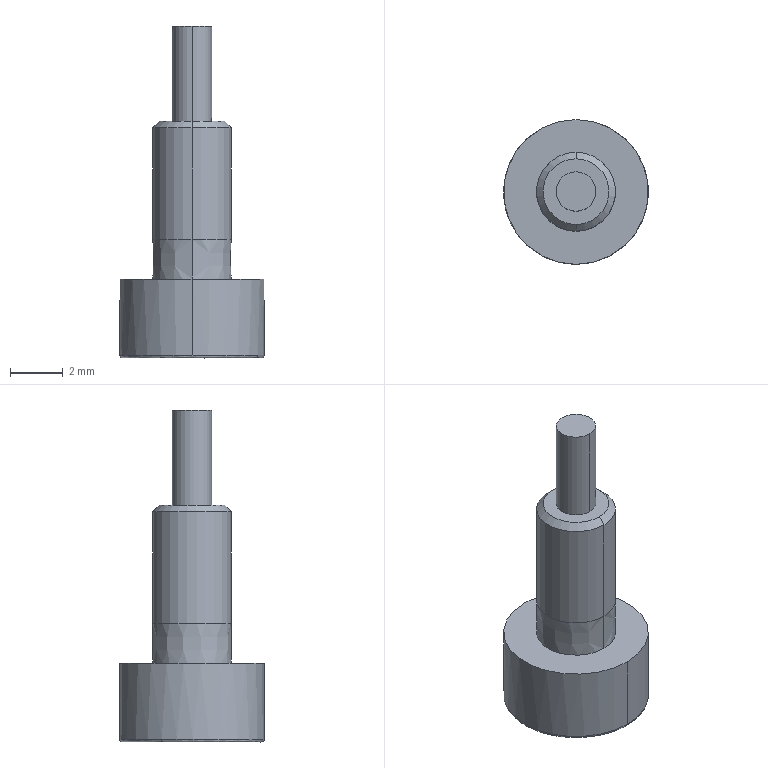Part | SolidWorks | features BaseBody 1 | 1 solid | 23 faces | box 5.5 x 5.5 x 12.613 mm | volume 112.754 mm3 | plane 11 | cylinder 6 | cone 4 | spline 2 | commonest cylinder face diameters 1.5 x2 3 x2 5.5 x2
STEP:
#1=CARTESIAN_POINT('',(583.23,-162.694,210.645));
#2=VERTEX_POINT('',#1);
#3=CARTESIAN_POINT('',(585.728,-166.593,210.645));
#4=VERTEX_POINT('',#3);
#5=CARTESIAN_POINT('',(585.728,-163.843,210.645));
#6=DIRECTION('',(0.000000001,-0.000000003,1.));
#7=DIRECTION('',(0.,-1.,-0.000000003));
#8=AXIS2_PLACEMENT_3D('',#5,#6,#7);
#9=CIRCLE('',#8,2.75);
#10=EDGE_CURVE('',#2,#4,#9,.T.);
#11=ORIENTED_EDGE('',*,*,#10,.F.);
#12=CARTESIAN_POINT('',(583.321,-162.735,210.545));
#13=VERTEX_POINT('',#12);
#14=CARTESIAN_POINT('',(583.321,-162.735,210.645));
#15=DIRECTION('',(-0.4179,-0.9085,-0.000000003));
#16=DIRECTION('',(-0.9085,0.4179,0.000000002));
#17=AXIS2_PLACEMENT_3D('',#14,#15,#16);
#18=CIRCLE('',#17,0.1);
#19=EDGE_CURVE('',#2,#13,#18,.T.);
#20=ORIENTED_EDGE('',*,*,#19,.T.);
#21=CARTESIAN_POINT('',(588.136,-164.951,210.545));
#22=VERTEX_POINT('',#21);
#23=CARTESIAN_POINT('',(583.321,-162.735,210.545));
#24=CARTESIAN_POINT('',(581.106,-167.55,210.545));
#25=CARTESIAN_POINT('',(585.921,-169.765,210.545));
#26=CARTESIAN_POINT('',(588.136,-164.951,210.545));
#27=(BOUNDED_CURVE()B_SPLINE_CURVE(3,(#23,#24,#25,#26),.UNSPECIFIED.,.F.,.T.)B_SPLINE_CURVE_WITH_KNOTS((4,4),(0.,1.),.UNSPECIFIED.)CURVE()GEOMETRIC_REPRESENTATION_ITEM()RATIONAL_B_SPLINE_CURVE((1.,0.3333,0.3333,1.))REPRESENTATION_ITEM(''));
#28=EDGE_CURVE('',#13,#22,#27,.T.);
#29=ORIENTED_EDGE('',*,*,#28,.T.);
#30=CARTESIAN_POINT('',(588.227,-164.992,210.645));
#31=VERTEX_POINT('',#30);
#32=CARTESIAN_POINT('',(588.136,-164.951,210.645));
#33=DIRECTION('',(0.4179,0.9085,0.000000003));
#34=DIRECTION('',(0.9085,-0.4179,-0.000000002));
#35=AXIS2_PLACEMENT_3D('',#32,#33,#34);
#36=CIRCLE('',#35,0.1);
#37=EDGE_CURVE('',#31,#22,#36,.T.);
#38=ORIENTED_EDGE('',*,*,#37,.F.);
#39=CARTESIAN_POINT('',(585.728,-163.843,210.645));
#40=DIRECTION('',(0.000000001,-0.000000003,1.));
#41=DIRECTION('',(0.,-1.,-0.000000003));
#42=AXIS2_PLACEMENT_3D('',#39,#40,#41);
#43=CIRCLE('',#42,2.75);
#44=EDGE_CURVE('',#4,#31,#43,.T.);
#45=ORIENTED_EDGE('',*,*,#44,.F.);
#46=EDGE_LOOP('',(#11,#20,#29,#38,#45));
#47=FACE_OUTER_BOUND('',#46,.T.);
#48=CARTESIAN_POINT('',(583.23,-162.694,210.645));
#49=CARTESIAN_POINT('',(580.931,-167.69,210.645));
#50=CARTESIAN_POINT('',(585.928,-169.989,210.645));
#51=CARTESIAN_POINT('',(588.227,-164.992,210.645));
#52=CARTESIAN_POINT('',(583.23,-162.694,210.586));
#53=CARTESIAN_POINT('',(580.931,-167.69,210.586));
#54=CARTESIAN_POINT('',(585.928,-169.989,210.586));
#55=CARTESIAN_POINT('',(588.227,-164.992,210.586));
#56=CARTESIAN_POINT('',(583.268,-162.711,210.545));
#57=CARTESIAN_POINT('',(581.003,-167.632,210.545));
#58=CARTESIAN_POINT('',(585.925,-169.896,210.545));
#59=CARTESIAN_POINT('',(588.189,-164.975,210.545));
#60=CARTESIAN_POINT('',(583.321,-162.735,210.545));
#61=CARTESIAN_POINT('',(581.106,-167.55,210.545));
#62=CARTESIAN_POINT('',(585.921,-169.765,210.545));
#63=CARTESIAN_POINT('',(588.136,-164.951,210.545));
#64=(BOUNDED_SURFACE()B_SPLINE_SURFACE(3,3,((#48,#49,#50,#51),(#52,#53,#54,#55),(#56,#57,#58,#59),(#60,#61,#62,#63)),.UNSPECIFIED.,.F.,.F.,.T.)B_SPLINE_SURFACE_WITH_KNOTS((4,4),(4,4),(0.,1.),(0.,1.),.UNSPECIFIED.)GEOMETRIC_REPRESENTATION_ITEM()RATIONAL_B_SPLINE_SURFACE(((1.,0.3333,0.3333,1.),(0.8047,0.2682,0.2682,0.8047),(0.8047,0.2682,0.2682,0.8047),(1.,0.3333,0.3333,1.)))REPRESENTATION_ITEM('')SURFACE());
#65=ADVANCED_FACE('',(#47),#64,.T.);
#66=ORIENTED_EDGE('',*,*,#44,.T.);
#67=CARTESIAN_POINT('',(585.728,-161.093,210.645));
#68=VERTEX_POINT('',#67);
#69=CARTESIAN_POINT('',(585.728,-163.843,210.645));
#70=DIRECTION('',(0.000000001,-0.000000003,1.));
#71=DIRECTION('',(0.,-1.,-0.000000003));
#72=AXIS2_PLACEMENT_3D('',#69,#70,#71);
#73=CIRCLE('',#72,2.75);
#74=EDGE_CURVE('',#31,#68,#73,.T.);
#75=ORIENTED_EDGE('',*,*,#74,.T.);
#76=CARTESIAN_POINT('',(585.728,-161.093,213.545));
#77=VERTEX_POINT('',#76);
#78=CARTESIAN_POINT('',(585.728,-161.093,212.095));
#79=DIRECTION('',(0.000000001,-0.000000003,1.));
#80=VECTOR('',#79,1000.);
#81=LINE('',#78,#80);
#82=EDGE_CURVE('',#68,#77,#81,.T.);
#83=ORIENTED_EDGE('',*,*,#82,.T.);
#84=CARTESIAN_POINT('',(585.728,-166.593,213.545));
#85=VERTEX_POINT('',#84);
#86=CARTESIAN_POINT('',(585.728,-163.843,213.545));
#87=DIRECTION('',(-0.000000001,0.000000003,-1.));
#88=DIRECTION('',(0.,-1.,-0.000000003));
#89=AXIS2_PLACEMENT_3D('',#86,#87,#88);
#90=CIRCLE('',#89,2.75);
#91=EDGE_CURVE('',#77,#85,#90,.T.);
#92=ORIENTED_EDGE('',*,*,#91,.T.);
#93=CARTESIAN_POINT('',(585.728,-166.593,212.095));
#94=DIRECTION('',(0.000000001,-0.000000003,1.));
#95=VECTOR('',#94,1000.);
#96=LINE('',#93,#95);
#97=EDGE_CURVE('',#4,#85,#96,.T.);
#98=ORIENTED_EDGE('',*,*,#97,.F.);
#99=EDGE_LOOP('',(#66,#75,#83,#92,#98));
#100=FACE_OUTER_BOUND('',#99,.T.);
#101=CARTESIAN_POINT('',(585.728,-163.843,212.095));
#102=DIRECTION('',(0.000000001,-0.000000003,1.));
#103=DIRECTION('',(0.,-1.,-0.000000003));
#104=AXIS2_PLACEMENT_3D('',#101,#102,#103);
#105=CYLINDRICAL_SURFACE('',#104,2.75);
#106=ADVANCED_FACE('',(#100),#105,.T.);
#107=CARTESIAN_POINT('',(585.728,-162.344,213.545));
#108=VERTEX_POINT('',#107);
#109=CARTESIAN_POINT('',(585.728,-165.342,213.545));
#110=VERTEX_POINT('',#109);
#111=CARTESIAN_POINT('',(585.728,-163.843,213.545));
#112=DIRECTION('',(-0.000000001,0.000000003,-1.));
#113=DIRECTION('',(0.,-1.,-0.000000003));
#114=AXIS2_PLACEMENT_3D('',#111,#112,#113);
#115=CIRCLE('',#114,1.499);
#116=EDGE_CURVE('',#108,#110,#115,.T.);
#117=ORIENTED_EDGE('',*,*,#116,.F.);
#118=CARTESIAN_POINT('',(585.728,-162.343,215.045));
#119=VERTEX_POINT('',#118);
#120=CARTESIAN_POINT('',(585.728,-162.343,215.045));
#121=DIRECTION('',(0.000000001,0.0005,1.));
#122=VECTOR('',#121,1000.);
#123=LINE('',#120,#122);
#124=EDGE_CURVE('',#108,#119,#123,.T.);
#125=ORIENTED_EDGE('',*,*,#124,.T.);
#126=CARTESIAN_POINT('',(585.728,-165.343,215.045));
#127=VERTEX_POINT('',#126);
#128=CARTESIAN_POINT('',(585.728,-163.843,215.045));
#129=DIRECTION('',(-0.000000001,0.000000003,-1.));
#130=DIRECTION('',(0.9085,-0.4179,-0.000000002));
#131=AXIS2_PLACEMENT_3D('',#128,#129,#130);
#132=CIRCLE('',#131,1.5);
#133=EDGE_CURVE('',#119,#127,#132,.T.);
#134=ORIENTED_EDGE('',*,*,#133,.T.);
#135=CARTESIAN_POINT('',(585.728,-165.343,215.045));
#136=DIRECTION('',(0.000000001,-0.0005,1.));
#137=VECTOR('',#136,1000.);
#138=LINE('',#135,#137);
#139=EDGE_CURVE('',#110,#127,#138,.T.);
#140=ORIENTED_EDGE('',*,*,#139,.F.);
#141=EDGE_LOOP('',(#117,#125,#134,#140));
#142=FACE_OUTER_BOUND('',#141,.T.);
#143=CARTESIAN_POINT('',(585.728,-163.843,215.045));
#144=DIRECTION('',(0.000000001,-0.000000003,1.));
#145=DIRECTION('',(0.,-1.,-0.000000003));
#146=AXIS2_PLACEMENT_3D('',#143,#144,#145);
#147=CONICAL_SURFACE('',#146,1.5,0.0005);
#148=ADVANCED_FACE('',(#142),#147,.T.);
#149=ORIENTED_EDGE('',*,*,#133,.F.);
#150=CARTESIAN_POINT('',(585.728,-162.343,219.295));
#151=VERTEX_POINT('',#150);
#152=CARTESIAN_POINT('',(585.728,-162.343,217.17));
#153=DIRECTION('',(0.000000001,-0.000000003,1.));
#154=VECTOR('',#153,1000.);
#155=LINE('',#152,#154);
#156=EDGE_CURVE('',#119,#151,#155,.T.);
#157=ORIENTED_EDGE('',*,*,#156,.T.);
#158=CARTESIAN_POINT('',(585.728,-165.343,219.295));
#159=VERTEX_POINT('',#158);
#160=CARTESIAN_POINT('',(585.728,-163.843,219.295));
#161=DIRECTION('',(-0.000000001,0.000000003,-1.));
#162=DIRECTION('',(0.,-1.,-0.000000003));
#163=AXIS2_PLACEMENT_3D('',#160,#161,#162);
#164=CIRCLE('',#163,1.5);
#165=EDGE_CURVE('',#151,#159,#164,.T.);
#166=ORIENTED_EDGE('',*,*,#165,.T.);
#167=CARTESIAN_POINT('',(585.728,-165.343,217.17));
#168=DIRECTION('',(0.000000001,-0.000000003,1.));
#169=VECTOR('',#168,1000.);
#170=LINE('',#167,#169);
#171=EDGE_CURVE('',#127,#159,#170,.T.);
#172=ORIENTED_EDGE('',*,*,#171,.F.);
#173=EDGE_LOOP('',(#149,#157,#166,#172));
#174=FACE_OUTER_BOUND('',#173,.T.);
#175=CARTESIAN_POINT('',(585.728,-163.843,217.17));
#176=DIRECTION('',(0.000000001,-0.000000003,1.));
#177=DIRECTION('',(0.,-1.,-0.000000003));
#178=AXIS2_PLACEMENT_3D('',#175,#176,#177);
#179=CYLINDRICAL_SURFACE('',#178,1.5);
#180=ADVANCED_FACE('',(#174),#179,.T.);
#181=CARTESIAN_POINT('',(585.728,-162.593,219.545));
#182=VERTEX_POINT('',#181);
#183=CARTESIAN_POINT('',(585.728,-165.093,219.545));
#184=VERTEX_POINT('',#183);
#185=CARTESIAN_POINT('',(585.728,-163.843,219.545));
#186=DIRECTION('',(-0.000000001,0.000000003,-1.));
#187=DIRECTION('',(0.,1.,0.000000003));
#188=AXIS2_PLACEMENT_3D('',#185,#186,#187);
#189=CIRCLE('',#188,1.25);
#190=EDGE_CURVE('',#182,#184,#189,.T.);
#191=ORIENTED_EDGE('',*,*,#190,.T.);
#192=CARTESIAN_POINT('',(585.728,-165.343,219.295));
#193=DIRECTION('',(-0.000000001,-0.7071,-0.7071));
#194=VECTOR('',#193,1000.);
#195=LINE('',#192,#194);
#196=EDGE_CURVE('',#184,#159,#195,.T.);
#197=ORIENTED_EDGE('',*,*,#196,.T.);
#198=ORIENTED_EDGE('',*,*,#165,.F.);
#199=CARTESIAN_POINT('',(585.728,-162.343,219.295));
#200=DIRECTION('',(-0.000000001,0.7071,-0.7071));
#201=VECTOR('',#200,1000.);
#202=LINE('',#199,#201);
#203=EDGE_CURVE('',#182,#151,#202,.T.);
#204=ORIENTED_EDGE('',*,*,#203,.F.);
#205=EDGE_LOOP('',(#191,#197,#198,#204));
#206=FACE_OUTER_BOUND('',#205,.T.);
#207=CARTESIAN_POINT('',(585.728,-163.843,219.295));
#208=DIRECTION('',(-0.000000001,0.000000003,-1.));
#209=DIRECTION('',(0.,1.,0.000000003));
#210=AXIS2_PLACEMENT_3D('',#207,#208,#209);
#211=CONICAL_SURFACE('',#210,1.5,0.7854);
#212=ADVANCED_FACE('',(#206),#211,.T.);
#213=CARTESIAN_POINT('',(585.728,-163.093,223.158));
#214=VERTEX_POINT('',#213);
#215=CARTESIAN_POINT('',(585.728,-164.593,223.158));
#216=VERTEX_POINT('',#215);
#217=CARTESIAN_POINT('',(585.728,-163.843,223.158));
#218=DIRECTION('',(-0.000000001,0.000000003,-1.));
#219=DIRECTION('',(0.,1.,0.000000003));
#220=AXIS2_PLACEMENT_3D('',#217,#218,#219);
#221=CIRCLE('',#220,0.75);
#222=EDGE_CURVE('',#214,#216,#221,.T.);
#223=ORIENTED_EDGE('',*,*,#222,.T.);
#224=CARTESIAN_POINT('',(585.728,-164.593,219.545));
#225=VERTEX_POINT('',#224);
#226=CARTESIAN_POINT('',(585.728,-164.593,219.545));
#227=DIRECTION('',(-0.000000001,0.000000003,-1.));
#228=VECTOR('',#227,1000.);
#229=LINE('',#226,#228);
#230=EDGE_CURVE('',#216,#225,#229,.T.);
#231=ORIENTED_EDGE('',*,*,#230,.T.);
#232=CARTESIAN_POINT('',(585.728,-163.093,219.545));
#233=VERTEX_POINT('',#232);
#234=CARTESIAN_POINT('',(585.728,-163.843,219.545));
#235=DIRECTION('',(-0.000000001,0.000000003,-1.));
#236=DIRECTION('',(0.,1.,0.000000003));
#237=AXIS2_PLACEMENT_3D('',#234,#235,#236);
#238=CIRCLE('',#237,0.75);
#239=EDGE_CURVE('',#233,#225,#238,.T.);
#240=ORIENTED_EDGE('',*,*,#239,.F.);
#241=CARTESIAN_POINT('',(585.728,-163.093,219.545));
#242=DIRECTION('',(-0.000000001,0.000000003,-1.));
#243=VECTOR('',#242,1000.);
#244=LINE('',#241,#243);
#245=EDGE_CURVE('',#214,#233,#244,.T.);
#246=ORIENTED_EDGE('',*,*,#245,.F.);
#247=EDGE_LOOP('',(#223,#231,#240,#246));
#248=FACE_OUTER_BOUND('',#247,.T.);
#249=CARTESIAN_POINT('',(585.728,-163.843,219.545));
#250=DIRECTION('',(-0.000000001,0.000000003,-1.));
#251=DIRECTION('',(0.,1.,0.000000003));
#252=AXIS2_PLACEMENT_3D('',#249,#250,#251);
#253=CYLINDRICAL_SURFACE('',#252,0.75);
#254=ADVANCED_FACE('',(#248),#253,.T.);
#255=ORIENTED_EDGE('',*,*,#82,.F.);
#256=CARTESIAN_POINT('',(585.728,-163.843,210.645));
#257=DIRECTION('',(0.000000001,-0.000000003,1.));
#258=DIRECTION('',(0.,-1.,-0.000000003));
#259=AXIS2_PLACEMENT_3D('',#256,#257,#258);
#260=CIRCLE('',#259,2.75);
#261=EDGE_CURVE('',#68,#2,#260,.T.);
#262=ORIENTED_EDGE('',*,*,#261,.T.);
#263=ORIENTED_EDGE('',*,*,#10,.T.);
#264=ORIENTED_EDGE('',*,*,#97,.T.);
#265=CARTESIAN_POINT('',(585.728,-163.843,213.545));
#266=DIRECTION('',(-0.000000001,0.000000003,-1.));
#267=DIRECTION('',(0.,-1.,-0.000000003));
#268=AXIS2_PLACEMENT_3D('',#265,#266,#267);
#269=CIRCLE('',#268,2.75);
#270=EDGE_CURVE('',#85,#77,#269,.T.);
#271=ORIENTED_EDGE('',*,*,#270,.T.);
#272=EDGE_LOOP('',(#255,#262,#263,#264,#271));
#273=FACE_OUTER_BOUND('',#272,.T.);
#274=CARTESIAN_POINT('',(585.728,-163.843,212.095));
#275=DIRECTION('',(0.000000001,-0.000000003,1.));
#276=DIRECTION('',(0.,-1.,-0.000000003));
#277=AXIS2_PLACEMENT_3D('',#274,#275,#276);
#278=CYLINDRICAL_SURFACE('',#277,2.75);
#279=ADVANCED_FACE('',(#273),#278,.T.);
#280=ORIENTED_EDGE('',*,*,#19,.F.);
#281=ORIENTED_EDGE('',*,*,#261,.F.);
#282=ORIENTED_EDGE('',*,*,#74,.F.);
#283=ORIENTED_EDGE('',*,*,#37,.T.);
#284=CARTESIAN_POINT('',(583.321,-162.735,210.545));
#285=CARTESIAN_POINT('',(583.391,-162.582,210.545));
#286=CARTESIAN_POINT('',(583.516,-162.367,210.545));
#287=CARTESIAN_POINT('',(583.695,-162.139,210.545));
#288=CARTESIAN_POINT('',(583.794,-162.031,210.545));
#289=CARTESIAN_POINT('',(583.838,-161.986,210.545));
#290=CARTESIAN_POINT('',(583.867,-161.956,210.545));
#291=CARTESIAN_POINT('',(583.881,-161.943,210.545));
#292=CARTESIAN_POINT('',(584.162,-161.674,210.545));
#293=CARTESIAN_POINT('',(584.466,-161.484,210.545));
#294=CARTESIAN_POINT('',(584.98,-161.294,210.545));
#295=CARTESIAN_POINT('',(585.242,-161.226,210.545));
#296=CARTESIAN_POINT('',(585.554,-161.196,210.545));
#297=CARTESIAN_POINT('',(585.712,-161.192,210.545));
#298=CARTESIAN_POINT('',(585.781,-161.193,210.545));
#299=CARTESIAN_POINT('',(585.826,-161.195,210.545));
#300=CARTESIAN_POINT('',(585.851,-161.196,210.545));
#301=CARTESIAN_POINT('',(586.208,-161.215,210.545));
#302=CARTESIAN_POINT('',(586.53,-161.295,210.545));
#303=CARTESIAN_POINT('',(586.989,-161.506,210.545));
#304=CARTESIAN_POINT('',(587.204,-161.631,210.545));
#305=CARTESIAN_POINT('',(587.432,-161.81,210.545));
#306=CARTESIAN_POINT('',(587.54,-161.908,210.545));
#307=CARTESIAN_POINT('',(587.585,-161.952,210.545));
#308=CARTESIAN_POINT('',(587.615,-161.982,210.545));
#309=CARTESIAN_POINT('',(587.628,-161.996,210.545));
#310=CARTESIAN_POINT('',(587.897,-162.276,210.545));
#311=CARTESIAN_POINT('',(588.087,-162.581,210.545));
#312=CARTESIAN_POINT('',(588.277,-163.095,210.545));
#313=CARTESIAN_POINT('',(588.345,-163.357,210.545));
#314=CARTESIAN_POINT('',(588.376,-163.669,210.545));
#315=CARTESIAN_POINT('',(588.379,-163.827,210.545));
#316=CARTESIAN_POINT('',(588.378,-163.895,210.545));
#317=CARTESIAN_POINT('',(588.377,-163.941,210.545));
#318=CARTESIAN_POINT('',(588.375,-163.966,210.545));
#319=CARTESIAN_POINT('',(588.356,-164.323,210.545));
#320=CARTESIAN_POINT('',(588.277,-164.644,210.545));
#321=CARTESIAN_POINT('',(588.136,-164.951,210.545));
#322=B_SPLINE_CURVE_WITH_KNOTS('',3,(#284,#285,#286,#287,#288,#289,#290,#291,#292,#293,#294,#295,#296,#297,#298,#299,#300,#301,#302,#303,#304,#305,#306,#307,#308,#309,#310,#311,#312,#313,#314,#315,#316,#317,#318,#319,#320,#321),.UNSPECIFIED.,.F.,.F.,(4,1,1,1,2,2,2,1,1,1,2,2,2,1,1,1,2,2,2,1,1,1,2,2,4),(0.,0.0625,0.09375,0.1094,0.1172,0.125,0.25,0.3125,0.3438,0.3594,0.3672,0.375,0.5,0.5625,0.5937,0.6094,0.6172,0.625,0.75,0.8125,0.8437,0.8594,0.8672,0.875,1.),.UNSPECIFIED.);
#323=EDGE_CURVE('',#13,#22,#322,.T.);
#324=ORIENTED_EDGE('',*,*,#323,.F.);
#325=EDGE_LOOP('',(#280,#281,#282,#283,#324));
#326=FACE_OUTER_BOUND('',#325,.T.);
#327=CARTESIAN_POINT('',(588.227,-164.992,210.645));
#328=CARTESIAN_POINT('',(590.525,-159.996,210.645));
#329=CARTESIAN_POINT('',(585.529,-157.697,210.645));
#330=CARTESIAN_POINT('',(583.23,-162.694,210.645));
#331=CARTESIAN_POINT('',(588.227,-164.992,210.586));
#332=CARTESIAN_POINT('',(590.525,-159.996,210.586));
#333=CARTESIAN_POINT('',(585.529,-157.697,210.586));
#334=CARTESIAN_POINT('',(583.23,-162.694,210.586));
#335=CARTESIAN_POINT('',(588.189,-164.975,210.545));
#336=CARTESIAN_POINT('',(590.453,-160.054,210.545));
#337=CARTESIAN_POINT('',(585.532,-157.79,210.545));
#338=CARTESIAN_POINT('',(583.268,-162.711,210.545));
#339=CARTESIAN_POINT('',(588.136,-164.951,210.545));
#340=CARTESIAN_POINT('',(590.351,-160.136,210.545));
#341=CARTESIAN_POINT('',(585.536,-157.921,210.545));
#342=CARTESIAN_POINT('',(583.321,-162.735,210.545));
#343=(BOUNDED_SURFACE()B_SPLINE_SURFACE(3,3,((#327,#328,#329,#330),(#331,#332,#333,#334),(#335,#336,#337,#338),(#339,#340,#341,#342)),.UNSPECIFIED.,.F.,.F.,.F.)B_SPLINE_SURFACE_WITH_KNOTS((4,4),(4,4),(0.,1.),(0.,1.),.UNSPECIFIED.)GEOMETRIC_REPRESENTATION_ITEM()RATIONAL_B_SPLINE_SURFACE(((1.,0.3333,0.3333,1.),(0.8047,0.2682,0.2682,0.8047),(0.8047,0.2682,0.2682,0.8047),(1.,0.3333,0.3333,1.)))REPRESENTATION_ITEM('')SURFACE());
#344=ADVANCED_FACE('',(#326),#343,.T.);
#345=CARTESIAN_POINT('',(585.728,-163.843,213.545));
#346=DIRECTION('',(-0.000000001,0.000000003,-1.));
#347=DIRECTION('',(0.,-1.,-0.000000003));
#348=AXIS2_PLACEMENT_3D('',#345,#346,#347);
#349=CIRCLE('',#348,1.499);
#350=EDGE_CURVE('',#110,#108,#349,.T.);
#351=ORIENTED_EDGE('',*,*,#350,.T.);
#352=ORIENTED_EDGE('',*,*,#116,.T.);
#353=EDGE_LOOP('',(#351,#352));
#354=FACE_BOUND('',#353,.T.);
#355=ORIENTED_EDGE('',*,*,#270,.F.);
#356=ORIENTED_EDGE('',*,*,#91,.F.);
#357=EDGE_LOOP('',(#355,#356));
#358=FACE_OUTER_BOUND('',#357,.T.);
#359=CARTESIAN_POINT('',(586.977,-164.418,213.545));
#360=DIRECTION('',(0.000000001,-0.000000003,1.));
#361=DIRECTION('',(0.,-1.,-0.000000003));
#362=AXIS2_PLACEMENT_3D('',#359,#360,#361);
#363=PLANE('',#362);
#364=ADVANCED_FACE('',(#354,#358),#363,.T.);
#365=ORIENTED_EDGE('',*,*,#28,.F.);
#366=ORIENTED_EDGE('',*,*,#323,.T.);
#367=EDGE_LOOP('',(#365,#366));
#368=FACE_OUTER_BOUND('',#367,.T.);
#369=CARTESIAN_POINT('',(585.595,-162.406,210.545));
#370=VERTEX_POINT('',#369);
#371=CARTESIAN_POINT('',(584.417,-163.24,210.545));
#372=VERTEX_POINT('',#371);
#373=CARTESIAN_POINT('',(585.595,-162.406,210.545));
#374=DIRECTION('',(-0.8162,-0.5778,-0.000000001));
#375=VECTOR('',#374,1000.);
#376=LINE('',#373,#375);
#377=EDGE_CURVE('',#370,#372,#376,.T.);
#378=ORIENTED_EDGE('',*,*,#377,.T.);
#379=CARTESIAN_POINT('',(584.55,-164.677,210.545));
#380=VERTEX_POINT('',#379);
#381=CARTESIAN_POINT('',(584.417,-163.24,210.545));
#382=DIRECTION('',(0.09229,-0.9957,-0.000000003));
#383=VECTOR('',#382,1000.);
#384=LINE('',#381,#383);
#385=EDGE_CURVE('',#372,#380,#384,.T.);
#386=ORIENTED_EDGE('',*,*,#385,.T.);
#387=CARTESIAN_POINT('',(585.861,-165.28,210.545));
#388=VERTEX_POINT('',#387);
#389=CARTESIAN_POINT('',(584.55,-164.677,210.545));
#390=DIRECTION('',(0.9085,-0.4179,-0.000000002));
#391=VECTOR('',#390,1000.);
#392=LINE('',#389,#391);
#393=EDGE_CURVE('',#380,#388,#392,.T.);
#394=ORIENTED_EDGE('',*,*,#393,.T.);
#395=CARTESIAN_POINT('',(587.039,-164.446,210.545));
#396=VERTEX_POINT('',#395);
#397=CARTESIAN_POINT('',(585.861,-165.28,210.545));
#398=DIRECTION('',(0.8162,0.5778,0.000000001));
#399=VECTOR('',#398,1000.);
#400=LINE('',#397,#399);
#401=EDGE_CURVE('',#388,#396,#400,.T.);
#402=ORIENTED_EDGE('',*,*,#401,.T.);
#403=CARTESIAN_POINT('',(586.906,-163.009,210.545));
#404=VERTEX_POINT('',#403);
#405=CARTESIAN_POINT('',(587.039,-164.446,210.545));
#406=DIRECTION('',(-0.09229,0.9957,0.000000003));
#407=VECTOR('',#406,1000.);
#408=LINE('',#405,#407);
#409=EDGE_CURVE('',#396,#404,#408,.T.);
#410=ORIENTED_EDGE('',*,*,#409,.T.);
#411=CARTESIAN_POINT('',(586.906,-163.009,210.545));
#412=DIRECTION('',(-0.9085,0.4179,0.000000002));
#413=VECTOR('',#412,1000.);
#414=LINE('',#411,#413);
#415=EDGE_CURVE('',#404,#370,#414,.T.);
#416=ORIENTED_EDGE('',*,*,#415,.T.);
#417=EDGE_LOOP('',(#378,#386,#394,#402,#410,#416));
#418=FACE_BOUND('',#417,.T.);
#419=CARTESIAN_POINT('',(586.932,-164.397,210.545));
#420=DIRECTION('',(-0.000000001,0.000000003,-1.));
#421=DIRECTION('',(0.,1.,0.000000003));
#422=AXIS2_PLACEMENT_3D('',#419,#420,#421);
#423=PLANE('',#422);
#424=ADVANCED_FACE('',(#368,#418),#423,.T.);
#425=ORIENTED_EDGE('',*,*,#124,.F.);
#426=ORIENTED_EDGE('',*,*,#350,.F.);
#427=ORIENTED_EDGE('',*,*,#139,.T.);
#428=CARTESIAN_POINT('',(585.728,-163.843,215.045));
#429=DIRECTION('',(-0.000000001,0.000000003,-1.));
#430=DIRECTION('',(0.9085,-0.4179,-0.000000002));
#431=AXIS2_PLACEMENT_3D('',#428,#429,#430);
#432=CIRCLE('',#431,1.5);
#433=EDGE_CURVE('',#127,#119,#432,.T.);
#434=ORIENTED_EDGE('',*,*,#433,.T.);
#435=EDGE_LOOP('',(#425,#426,#427,#434));
#436=FACE_OUTER_BOUND('',#435,.T.);
#437=CARTESIAN_POINT('',(585.728,-163.843,215.045));
#438=DIRECTION('',(0.000000001,-0.000000003,1.));
#439=DIRECTION('',(0.,-1.,-0.000000003));
#440=AXIS2_PLACEMENT_3D('',#437,#438,#439);
#441=CONICAL_SURFACE('',#440,1.5,0.0005);
#442=ADVANCED_FACE('',(#436),#441,.T.);
#443=CARTESIAN_POINT('',(584.55,-164.677,211.845));
#444=VERTEX_POINT('',#443);
#445=CARTESIAN_POINT('',(584.55,-164.677,210.545));
#446=DIRECTION('',(0.,0.,1.));
#447=VECTOR('',#446,1000.);
#448=LINE('',#445,#447);
#449=EDGE_CURVE('',#380,#444,#448,.T.);
#450=ORIENTED_EDGE('',*,*,#449,.F.);
#451=ORIENTED_EDGE('',*,*,#385,.F.);
#452=CARTESIAN_POINT('',(584.417,-163.24,211.845));
#453=VERTEX_POINT('',#452);
#454=CARTESIAN_POINT('',(584.417,-163.24,210.545));
#455=DIRECTION('',(0.,0.,-1.));
#456=VECTOR('',#455,1000.);
#457=LINE('',#454,#456);
#458=EDGE_CURVE('',#453,#372,#457,.T.);
#459=ORIENTED_EDGE('',*,*,#458,.F.);
#460=CARTESIAN_POINT('',(584.55,-164.677,211.845));
#461=DIRECTION('',(-0.09229,0.9957,0.));
#462=VECTOR('',#461,1000.);
#463=LINE('',#460,#462);
#464=EDGE_CURVE('',#444,#453,#463,.T.);
#465=ORIENTED_EDGE('',*,*,#464,.F.);
#466=EDGE_LOOP('',(#450,#451,#459,#465));
#467=FACE_OUTER_BOUND('',#466,.T.);
#468=CARTESIAN_POINT('',(584.55,-164.677,210.545));
#469=DIRECTION('',(-0.9957,-0.09229,0.));
#470=DIRECTION('',(0.09229,-0.9957,0.));
#471=AXIS2_PLACEMENT_3D('',#468,#469,#470);
#472=PLANE('',#471);
#473=ADVANCED_FACE('',(#467),#472,.F.);
#474=ORIENTED_EDGE('',*,*,#458,.T.);
#475=ORIENTED_EDGE('',*,*,#377,.F.);
#476=CARTESIAN_POINT('',(585.595,-162.406,211.845));
#477=VERTEX_POINT('',#476);
#478=CARTESIAN_POINT('',(585.595,-162.406,210.545));
#479=DIRECTION('',(-0.000000002,0.000000003,-1.));
#480=VECTOR('',#479,1000.);
#481=LINE('',#478,#480);
#482=EDGE_CURVE('',#477,#370,#481,.T.);
#483=ORIENTED_EDGE('',*,*,#482,.F.);
#484=CARTESIAN_POINT('',(584.417,-163.24,211.845));
#485=DIRECTION('',(0.8162,0.5778,0.));
#486=VECTOR('',#485,1000.);
#487=LINE('',#484,#486);
#488=EDGE_CURVE('',#453,#477,#487,.T.);
#489=ORIENTED_EDGE('',*,*,#488,.F.);
#490=EDGE_LOOP('',(#474,#475,#483,#489));
#491=FACE_OUTER_BOUND('',#490,.T.);
#492=CARTESIAN_POINT('',(584.417,-163.24,210.545));
#493=DIRECTION('',(-0.5778,0.8162,0.000000003));
#494=DIRECTION('',(-0.8162,-0.5778,0.));
#495=AXIS2_PLACEMENT_3D('',#492,#493,#494);
#496=PLANE('',#495);
#497=ADVANCED_FACE('',(#491),#496,.F.);
#498=ORIENTED_EDGE('',*,*,#482,.T.);
#499=ORIENTED_EDGE('',*,*,#415,.F.);
#500=CARTESIAN_POINT('',(586.906,-163.009,211.845));
#501=VERTEX_POINT('',#500);
#502=CARTESIAN_POINT('',(586.906,-163.009,210.545));
#503=DIRECTION('',(0.000000001,0.000000002,-1.));
#504=VECTOR('',#503,1000.);
#505=LINE('',#502,#504);
#506=EDGE_CURVE('',#501,#404,#505,.T.);
#507=ORIENTED_EDGE('',*,*,#506,.F.);
#508=CARTESIAN_POINT('',(585.595,-162.406,211.845));
#509=DIRECTION('',(0.9085,-0.4179,0.));
#510=VECTOR('',#509,1000.);
#511=LINE('',#508,#510);
#512=EDGE_CURVE('',#477,#501,#511,.T.);
#513=ORIENTED_EDGE('',*,*,#512,.F.);
#514=EDGE_LOOP('',(#498,#499,#507,#513));
#515=FACE_OUTER_BOUND('',#514,.T.);
#516=CARTESIAN_POINT('',(585.595,-162.406,210.545));
#517=DIRECTION('',(0.4179,0.9085,0.000000003));
#518=DIRECTION('',(-0.9085,0.4179,0.));
#519=AXIS2_PLACEMENT_3D('',#516,#517,#518);
#520=PLANE('',#519);
#521=ADVANCED_FACE('',(#515),#520,.F.);
#522=ORIENTED_EDGE('',*,*,#506,.T.);
#523=ORIENTED_EDGE('',*,*,#409,.F.);
#524=CARTESIAN_POINT('',(587.039,-164.446,211.845));
#525=VERTEX_POINT('',#524);
#526=CARTESIAN_POINT('',(587.039,-164.446,210.545));
#527=DIRECTION('',(0.,0.,-1.));
#528=VECTOR('',#527,1000.);
#529=LINE('',#526,#528);
#530=EDGE_CURVE('',#525,#396,#529,.T.);
#531=ORIENTED_EDGE('',*,*,#530,.F.);
#532=CARTESIAN_POINT('',(586.906,-163.009,211.845));
#533=DIRECTION('',(0.09229,-0.9957,0.));
#534=VECTOR('',#533,1000.);
#535=LINE('',#532,#534);
#536=EDGE_CURVE('',#501,#525,#535,.T.);
#537=ORIENTED_EDGE('',*,*,#536,.F.);
#538=EDGE_LOOP('',(#522,#523,#531,#537));
#539=FACE_OUTER_BOUND('',#538,.T.);
#540=CARTESIAN_POINT('',(586.906,-163.009,210.545));
#541=DIRECTION('',(0.9957,0.09229,0.));
#542=DIRECTION('',(-0.09229,0.9957,0.));
#543=AXIS2_PLACEMENT_3D('',#540,#541,#542);
#544=PLANE('',#543);
#545=ADVANCED_FACE('',(#539),#544,.F.);
#546=ORIENTED_EDGE('',*,*,#530,.T.);
#547=ORIENTED_EDGE('',*,*,#401,.F.);
#548=CARTESIAN_POINT('',(585.861,-165.28,211.845));
#549=VERTEX_POINT('',#548);
#550=CARTESIAN_POINT('',(585.861,-165.28,210.545));
#551=DIRECTION('',(-0.000000002,0.000000003,-1.));
#552=VECTOR('',#551,1000.);
#553=LINE('',#550,#552);
#554=EDGE_CURVE('',#549,#388,#553,.T.);
#555=ORIENTED_EDGE('',*,*,#554,.F.);
#556=CARTESIAN_POINT('',(587.039,-164.446,211.845));
#557=DIRECTION('',(-0.8162,-0.5778,0.));
#558=VECTOR('',#557,1000.);
#559=LINE('',#556,#558);
#560=EDGE_CURVE('',#525,#549,#559,.T.);
#561=ORIENTED_EDGE('',*,*,#560,.F.);
#562=EDGE_LOOP('',(#546,#547,#555,#561));
#563=FACE_OUTER_BOUND('',#562,.T.);
#564=CARTESIAN_POINT('',(587.039,-164.446,210.545));
#565=DIRECTION('',(0.5778,-0.8162,-0.000000003));
#566=DIRECTION('',(0.8162,0.5778,0.));
#567=AXIS2_PLACEMENT_3D('',#564,#565,#566);
#568=PLANE('',#567);
#569=ADVANCED_FACE('',(#563),#568,.F.);
#570=ORIENTED_EDGE('',*,*,#554,.T.);
#571=ORIENTED_EDGE('',*,*,#393,.F.);
#572=ORIENTED_EDGE('',*,*,#449,.T.);
#573=CARTESIAN_POINT('',(585.861,-165.28,211.845));
#574=DIRECTION('',(-0.9085,0.4179,0.));
#575=VECTOR('',#574,1000.);
#576=LINE('',#573,#575);
#577=EDGE_CURVE('',#549,#444,#576,.T.);
#578=ORIENTED_EDGE('',*,*,#577,.F.);
#579=EDGE_LOOP('',(#570,#571,#572,#578));
#580=FACE_OUTER_BOUND('',#579,.T.);
#581=CARTESIAN_POINT('',(585.861,-165.28,210.545));
#582=DIRECTION('',(-0.4179,-0.9085,-0.000000003));
#583=DIRECTION('',(0.9085,-0.4179,0.));
#584=AXIS2_PLACEMENT_3D('',#581,#582,#583);
#585=PLANE('',#584);
#586=ADVANCED_FACE('',(#580),#585,.F.);
#587=ORIENTED_EDGE('',*,*,#156,.F.);
#588=ORIENTED_EDGE('',*,*,#433,.F.);
#589=ORIENTED_EDGE('',*,*,#171,.T.);
#590=CARTESIAN_POINT('',(585.728,-163.843,219.295));
#591=DIRECTION('',(-0.000000001,0.000000003,-1.));
#592=DIRECTION('',(0.,-1.,-0.000000003));
#593=AXIS2_PLACEMENT_3D('',#590,#591,#592);
#594=CIRCLE('',#593,1.5);
#595=EDGE_CURVE('',#159,#151,#594,.T.);
#596=ORIENTED_EDGE('',*,*,#595,.T.);
#597=EDGE_LOOP('',(#587,#588,#589,#596));
#598=FACE_OUTER_BOUND('',#597,.T.);
#599=CARTESIAN_POINT('',(585.728,-163.843,217.17));
#600=DIRECTION('',(0.000000001,-0.000000003,1.));
#601=DIRECTION('',(0.,-1.,-0.000000003));
#602=AXIS2_PLACEMENT_3D('',#599,#600,#601);
#603=CYLINDRICAL_SURFACE('',#602,1.5);
#604=ADVANCED_FACE('',(#598),#603,.T.);
#605=ORIENTED_EDGE('',*,*,#536,.T.);
#606=ORIENTED_EDGE('',*,*,#560,.T.);
#607=ORIENTED_EDGE('',*,*,#577,.T.);
#608=ORIENTED_EDGE('',*,*,#464,.T.);
#609=ORIENTED_EDGE('',*,*,#488,.T.);
#610=ORIENTED_EDGE('',*,*,#512,.T.);
#611=EDGE_LOOP('',(#605,#606,#607,#608,#609,#610));
#612=FACE_OUTER_BOUND('',#611,.T.);
#613=CARTESIAN_POINT('',(585.728,-163.843,211.845));
#614=DIRECTION('',(-0.000000001,0.000000003,-1.));
#615=DIRECTION('',(0.,1.,0.000000003));
#616=AXIS2_PLACEMENT_3D('',#613,#614,#615);
#617=PLANE('',#616);
#618=ADVANCED_FACE('',(#612),#617,.T.);
#619=ORIENTED_EDGE('',*,*,#196,.F.);
#620=CARTESIAN_POINT('',(585.728,-163.843,219.545));
#621=DIRECTION('',(-0.000000001,0.000000003,-1.));
#622=DIRECTION('',(0.,1.,0.000000003));
#623=AXIS2_PLACEMENT_3D('',#620,#621,#622);
#624=CIRCLE('',#623,1.25);
#625=EDGE_CURVE('',#184,#182,#624,.T.);
#626=ORIENTED_EDGE('',*,*,#625,.T.);
#627=ORIENTED_EDGE('',*,*,#203,.T.);
#628=ORIENTED_EDGE('',*,*,#595,.F.);
#629=EDGE_LOOP('',(#619,#626,#627,#628));
#630=FACE_OUTER_BOUND('',#629,.T.);
#631=CARTESIAN_POINT('',(585.728,-163.843,219.295));
#632=DIRECTION('',(-0.000000001,0.000000003,-1.));
#633=DIRECTION('',(0.,1.,0.000000003));
#634=AXIS2_PLACEMENT_3D('',#631,#632,#633);
#635=CONICAL_SURFACE('',#634,1.5,0.7854);
#636=ADVANCED_FACE('',(#630),#635,.T.);
#637=ORIENTED_EDGE('',*,*,#190,.F.);
#638=ORIENTED_EDGE('',*,*,#625,.F.);
#639=EDGE_LOOP('',(#637,#638));
#640=FACE_OUTER_BOUND('',#639,.T.);
#641=ORIENTED_EDGE('',*,*,#239,.T.);
#642=CARTESIAN_POINT('',(585.728,-163.843,219.545));
#643=DIRECTION('',(-0.000000001,0.000000003,-1.));
#644=DIRECTION('',(0.,1.,0.000000003));
#645=AXIS2_PLACEMENT_3D('',#642,#643,#644);
#646=CIRCLE('',#645,0.75);
#647=EDGE_CURVE('',#225,#233,#646,.T.);
#648=ORIENTED_EDGE('',*,*,#647,.T.);
#649=EDGE_LOOP('',(#641,#648));
#650=FACE_BOUND('',#649,.T.);
#651=CARTESIAN_POINT('',(586.296,-164.104,219.545));
#652=DIRECTION('',(0.000000001,-0.000000003,1.));
#653=DIRECTION('',(0.,-1.,-0.000000003));
#654=AXIS2_PLACEMENT_3D('',#651,#652,#653);
#655=PLANE('',#654);
#656=ADVANCED_FACE('',(#640,#650),#655,.T.);
#657=ORIENTED_EDGE('',*,*,#230,.F.);
#658=CARTESIAN_POINT('',(585.728,-163.843,223.158));
#659=DIRECTION('',(-0.000000001,0.000000003,-1.));
#660=DIRECTION('',(0.,1.,0.000000003));
#661=AXIS2_PLACEMENT_3D('',#658,#659,#660);
#662=CIRCLE('',#661,0.75);
#663=EDGE_CURVE('',#216,#214,#662,.T.);
#664=ORIENTED_EDGE('',*,*,#663,.T.);
#665=ORIENTED_EDGE('',*,*,#245,.T.);
#666=ORIENTED_EDGE('',*,*,#647,.F.);
#667=EDGE_LOOP('',(#657,#664,#665,#666));
#668=FACE_OUTER_BOUND('',#667,.T.);
#669=CARTESIAN_POINT('',(585.728,-163.843,219.545));
#670=DIRECTION('',(-0.000000001,0.000000003,-1.));
#671=DIRECTION('',(0.,1.,0.000000003));
#672=AXIS2_PLACEMENT_3D('',#669,#670,#671);
#673=CYLINDRICAL_SURFACE('',#672,0.75);
#674=ADVANCED_FACE('',(#668),#673,.T.);
#675=ORIENTED_EDGE('',*,*,#222,.F.);
#676=ORIENTED_EDGE('',*,*,#663,.F.);
#677=EDGE_LOOP('',(#675,#676));
#678=FACE_OUTER_BOUND('',#677,.T.);
#679=CARTESIAN_POINT('',(585.728,-163.843,223.158));
#680=DIRECTION('',(0.000000001,-0.000000003,1.));
#681=DIRECTION('',(0.,-1.,-0.000000003));
#682=AXIS2_PLACEMENT_3D('',#679,#680,#681);
#683=PLANE('',#682);
#684=ADVANCED_FACE('',(#678),#683,.T.);
#685=CLOSED_SHELL('',(#65,#106,#148,#180,#212,#254,#279,#344,#364,#424,#442,#473,#497,#521,#545,#569,#586,#604,#618,#636,#656,#674,#684));
#686=MANIFOLD_SOLID_BREP('',#685);
#687=CARTESIAN_POINT('',(0.,0.,0.));
#688=DIRECTION('',(0.,0.,1.));
#689=DIRECTION('',(1.,0.,0.));
#690=AXIS2_PLACEMENT_3D('',#687,#688,#689);
#691=(LENGTH_UNIT()NAMED_UNIT(*)SI_UNIT(.MILLI.,.METRE.));
#692=UNCERTAINTY_MEASURE_WITH_UNIT(LENGTH_MEASURE(0.00001),#691,'','');
#693=(NAMED_UNIT(*)PLANE_ANGLE_UNIT()SI_UNIT($,.RADIAN.));
#694=(NAMED_UNIT(*)SI_UNIT($,.STERADIAN.)SOLID_ANGLE_UNIT());
#695=(GEOMETRIC_REPRESENTATION_CONTEXT(3)GLOBAL_UNCERTAINTY_ASSIGNED_CONTEXT((#692))GLOBAL_UNIT_ASSIGNED_CONTEXT((#691,#693,#694))REPRESENTATION_CONTEXT('',''));
#696=ADVANCED_BREP_SHAPE_REPRESENTATION('',(#686,#690),#695);